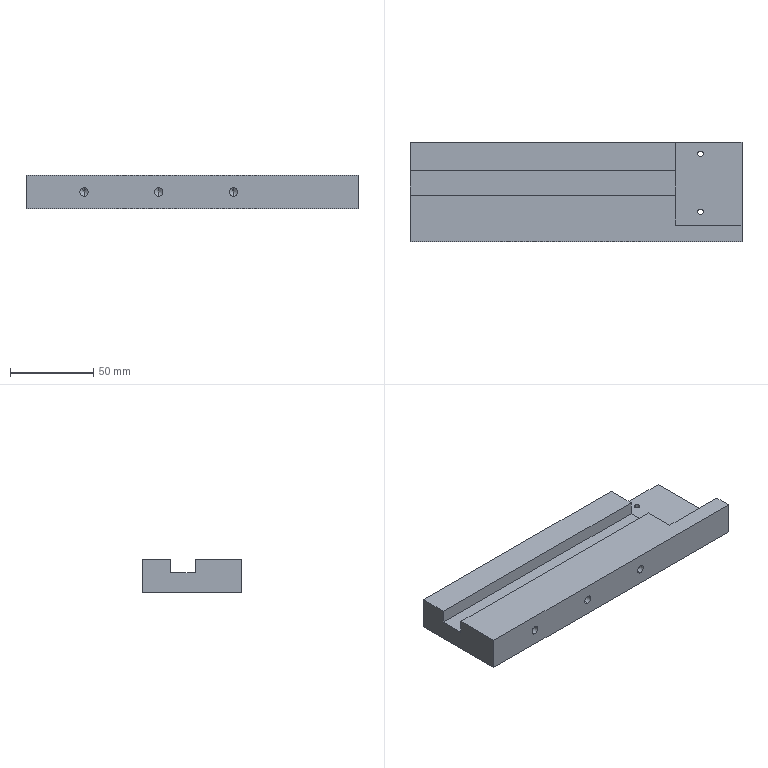Part | STEP file | 04-08 Rack support plate | 1 solid | 29 faces | box 200 x 60 x 20 mm | volume 189566 mm3 | plane 13 | cylinder 10 | cone 6 | commonest cylinder face diameters 5 x6 3.3 x4